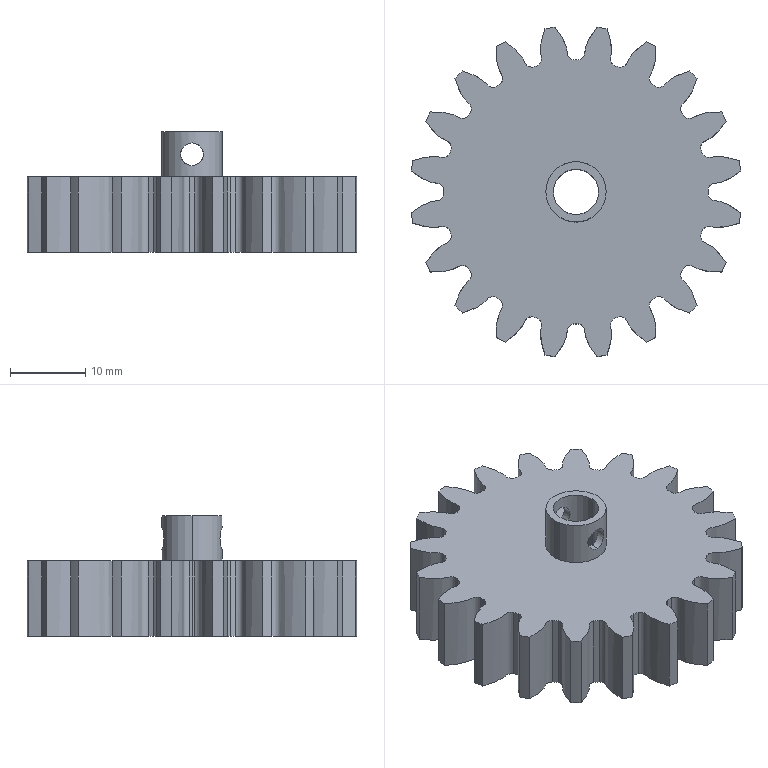Part | SolidWorks | features BaseBody 1 | 1 solid | 92 faces | box 43.654 x 43.654 x 16 mm | volume 12176 mm3 | cylinder 49 | spline 40 | plane 3 | commonest cylinder face diameters 35 x21 44 x20 3 x4 6 x2 8 x2